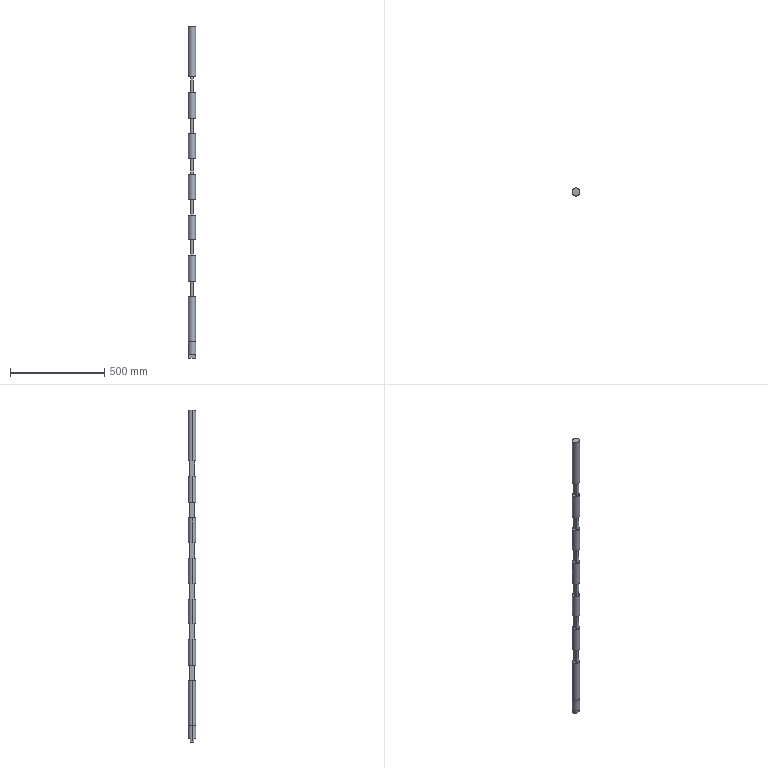Part | SolidWorks | 1 solid | 59 faces | box 40 x 40 x 1760 mm | volume 1700428 mm3 | plane 31 | cylinder 28 | commonest cylinder face diameters 30 x12 38 x10 40 x6